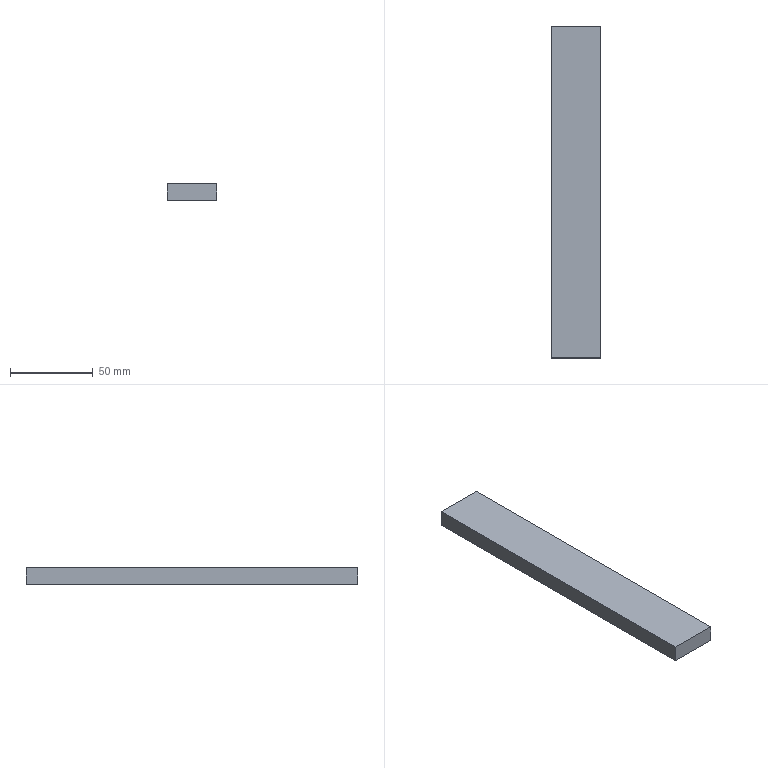Part | NX | features solid 2 | 1 solid | 6 faces | box 30 x 200 x 10 mm | volume 60000 mm3 | plane 6
STEP:
#1=CARTESIAN_POINT('',(-260.173,290.,-10.));
#2=VERTEX_POINT('',#1);
#3=CARTESIAN_POINT('',(-230.173,290.,-10.));
#4=VERTEX_POINT('',#3);
#5=CARTESIAN_POINT('',(-295.173,290.,-10.));
#6=DIRECTION('',(-1.,0.,0.));
#7=VECTOR('',#6,1000.);
#8=LINE('',#5,#7);
#9=EDGE_CURVE('',#2,#4,#8,.F.);
#10=ORIENTED_EDGE('',*,*,#9,.F.);
#11=CARTESIAN_POINT('',(-260.173,290.,-20.));
#12=VERTEX_POINT('',#11);
#13=CARTESIAN_POINT('',(-260.173,290.,0.));
#14=DIRECTION('',(0.,0.,1.));
#15=VECTOR('',#14,1000.);
#16=LINE('',#13,#15);
#17=EDGE_CURVE('',#2,#12,#16,.F.);
#18=ORIENTED_EDGE('',*,*,#17,.T.);
#19=CARTESIAN_POINT('',(-230.173,290.,-20.));
#20=VERTEX_POINT('',#19);
#21=CARTESIAN_POINT('',(-245.173,290.,-20.));
#22=DIRECTION('',(1.,0.,0.));
#23=VECTOR('',#22,1000.);
#24=LINE('',#21,#23);
#25=EDGE_CURVE('',#12,#20,#24,.T.);
#26=ORIENTED_EDGE('',*,*,#25,.T.);
#27=CARTESIAN_POINT('',(-230.173,290.,0.));
#28=DIRECTION('',(0.,0.,1.));
#29=VECTOR('',#28,1000.);
#30=LINE('',#27,#29);
#31=EDGE_CURVE('',#4,#20,#30,.F.);
#32=ORIENTED_EDGE('',*,*,#31,.F.);
#33=EDGE_LOOP('',(#10,#18,#26,#32));
#34=FACE_BOUND('',#33,.T.);
#35=CARTESIAN_POINT('',(-245.173,290.,0.));
#36=DIRECTION('',(0.,1.,0.));
#37=DIRECTION('',(0.,0.,-1.));
#38=AXIS2_PLACEMENT_3D('',#35,#36,#37);
#39=PLANE('',#38);
#40=ADVANCED_FACE('',(#34),#39,.F.);
#41=CARTESIAN_POINT('',(-230.173,490.,-20.));
#42=VERTEX_POINT('',#41);
#43=CARTESIAN_POINT('',(-230.173,490.,-20.));
#44=DIRECTION('',(0.,1.,0.));
#45=VECTOR('',#44,1000.);
#46=LINE('',#43,#45);
#47=EDGE_CURVE('',#42,#20,#46,.F.);
#48=ORIENTED_EDGE('',*,*,#47,.F.);
#49=CARTESIAN_POINT('',(-230.173,490.,-10.));
#50=VERTEX_POINT('',#49);
#51=CARTESIAN_POINT('',(-230.173,490.,0.));
#52=DIRECTION('',(0.,0.,1.));
#53=VECTOR('',#52,1000.);
#54=LINE('',#51,#53);
#55=EDGE_CURVE('',#42,#50,#54,.T.);
#56=ORIENTED_EDGE('',*,*,#55,.T.);
#57=CARTESIAN_POINT('',(-230.173,460.,-10.));
#58=DIRECTION('',(0.,-1.,0.));
#59=VECTOR('',#58,1000.);
#60=LINE('',#57,#59);
#61=EDGE_CURVE('',#50,#4,#60,.T.);
#62=ORIENTED_EDGE('',*,*,#61,.T.);
#63=ORIENTED_EDGE('',*,*,#31,.T.);
#64=EDGE_LOOP('',(#48,#56,#62,#63));
#65=FACE_BOUND('',#64,.T.);
#66=CARTESIAN_POINT('',(-230.173,490.,0.));
#67=DIRECTION('',(-1.,0.,0.));
#68=DIRECTION('',(0.,0.,1.));
#69=AXIS2_PLACEMENT_3D('',#66,#67,#68);
#70=PLANE('',#69);
#71=ADVANCED_FACE('',(#65),#70,.F.);
#72=CARTESIAN_POINT('',(-260.173,490.,-10.));
#73=VERTEX_POINT('',#72);
#74=CARTESIAN_POINT('',(-260.173,460.,-10.));
#75=DIRECTION('',(0.,-1.,0.));
#76=VECTOR('',#75,1000.);
#77=LINE('',#74,#76);
#78=EDGE_CURVE('',#73,#2,#77,.T.);
#79=ORIENTED_EDGE('',*,*,#78,.F.);
#80=CARTESIAN_POINT('',(-260.173,490.,-20.));
#81=VERTEX_POINT('',#80);
#82=CARTESIAN_POINT('',(-260.173,490.,-10.));
#83=DIRECTION('',(0.,0.,-1.));
#84=VECTOR('',#83,1000.);
#85=LINE('',#82,#84);
#86=EDGE_CURVE('',#73,#81,#85,.T.);
#87=ORIENTED_EDGE('',*,*,#86,.T.);
#88=CARTESIAN_POINT('',(-260.173,490.,-20.));
#89=DIRECTION('',(0.,1.,0.));
#90=VECTOR('',#89,1000.);
#91=LINE('',#88,#90);
#92=EDGE_CURVE('',#81,#12,#91,.F.);
#93=ORIENTED_EDGE('',*,*,#92,.T.);
#94=ORIENTED_EDGE('',*,*,#17,.F.);
#95=EDGE_LOOP('',(#79,#87,#93,#94));
#96=FACE_BOUND('',#95,.T.);
#97=CARTESIAN_POINT('',(-260.173,490.,0.));
#98=DIRECTION('',(-1.,0.,0.));
#99=DIRECTION('',(0.,0.,1.));
#100=AXIS2_PLACEMENT_3D('',#97,#98,#99);
#101=PLANE('',#100);
#102=ADVANCED_FACE('',(#96),#101,.T.);
#103=ORIENTED_EDGE('',*,*,#92,.F.);
#104=CARTESIAN_POINT('',(-374.173,490.,-20.));
#105=DIRECTION('',(1.,0.,0.));
#106=VECTOR('',#105,1000.);
#107=LINE('',#104,#106);
#108=EDGE_CURVE('',#81,#42,#107,.T.);
#109=ORIENTED_EDGE('',*,*,#108,.T.);
#110=ORIENTED_EDGE('',*,*,#47,.T.);
#111=ORIENTED_EDGE('',*,*,#25,.F.);
#112=EDGE_LOOP('',(#103,#109,#110,#111));
#113=FACE_BOUND('',#112,.T.);
#114=CARTESIAN_POINT('',(-374.173,460.,-20.));
#115=DIRECTION('',(0.,0.,1.));
#116=DIRECTION('',(1.,0.,0.));
#117=AXIS2_PLACEMENT_3D('',#114,#115,#116);
#118=PLANE('',#117);
#119=ADVANCED_FACE('',(#113),#118,.F.);
#120=CARTESIAN_POINT('',(-374.173,490.,-10.));
#121=DIRECTION('',(1.,0.,0.));
#122=VECTOR('',#121,1000.);
#123=LINE('',#120,#122);
#124=EDGE_CURVE('',#73,#50,#123,.T.);
#125=ORIENTED_EDGE('',*,*,#124,.F.);
#126=ORIENTED_EDGE('',*,*,#78,.T.);
#127=ORIENTED_EDGE('',*,*,#9,.T.);
#128=ORIENTED_EDGE('',*,*,#61,.F.);
#129=EDGE_LOOP('',(#125,#126,#127,#128));
#130=FACE_BOUND('',#129,.T.);
#131=CARTESIAN_POINT('',(-374.173,460.,-10.));
#132=DIRECTION('',(0.,0.,1.));
#133=DIRECTION('',(1.,0.,0.));
#134=AXIS2_PLACEMENT_3D('',#131,#132,#133);
#135=PLANE('',#134);
#136=ADVANCED_FACE('',(#130),#135,.T.);
#137=ORIENTED_EDGE('',*,*,#124,.T.);
#138=ORIENTED_EDGE('',*,*,#55,.F.);
#139=ORIENTED_EDGE('',*,*,#108,.F.);
#140=ORIENTED_EDGE('',*,*,#86,.F.);
#141=EDGE_LOOP('',(#137,#138,#139,#140));
#142=FACE_BOUND('',#141,.T.);
#143=CARTESIAN_POINT('',(-295.173,490.,-10.));
#144=DIRECTION('',(0.,-1.,0.));
#145=DIRECTION('',(1.,0.,0.));
#146=AXIS2_PLACEMENT_3D('',#143,#144,#145);
#147=PLANE('',#146);
#148=ADVANCED_FACE('',(#142),#147,.F.);
#149=CLOSED_SHELL('',(#40,#71,#102,#119,#136,#148));
#150=MANIFOLD_SOLID_BREP('',#149);
#151=(LENGTH_UNIT()NAMED_UNIT(*)SI_UNIT(.MILLI.,.METRE.));
#152=UNCERTAINTY_MEASURE_WITH_UNIT(LENGTH_MEASURE(0.00001),#151,'','');
#153=(NAMED_UNIT(*)PLANE_ANGLE_UNIT()SI_UNIT($,.RADIAN.));
#154=(NAMED_UNIT(*)SI_UNIT($,.STERADIAN.)SOLID_ANGLE_UNIT());
#155=(GEOMETRIC_REPRESENTATION_CONTEXT(3)GLOBAL_UNCERTAINTY_ASSIGNED_CONTEXT((#152))GLOBAL_UNIT_ASSIGNED_CONTEXT((#151,#153,#154))REPRESENTATION_CONTEXT('',''));
#156=ADVANCED_BREP_SHAPE_REPRESENTATION('',(#150),#155);